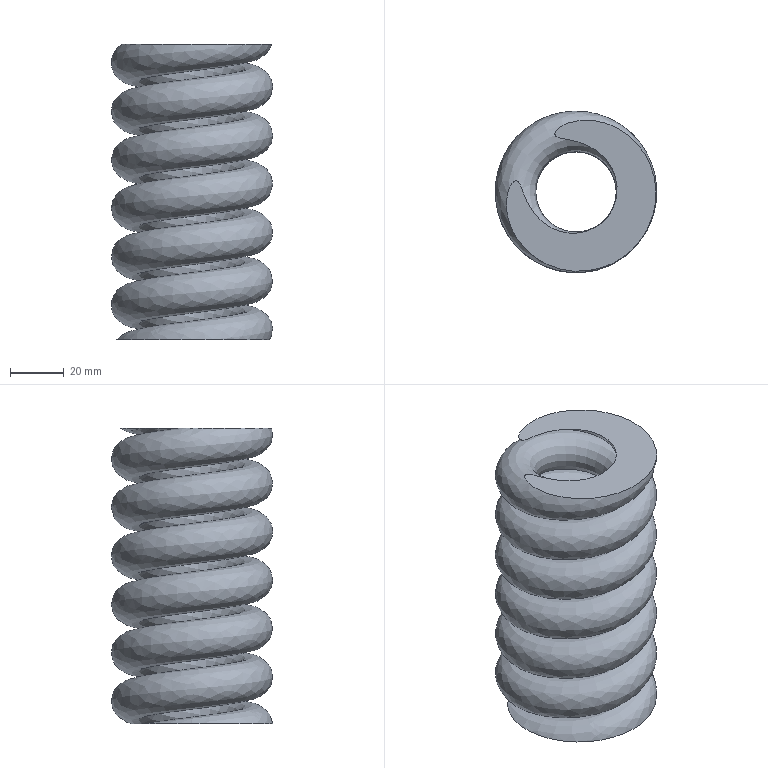Part | NX | features solid 2 | 1 solid | 3 faces | box 60 x 60 x 110 mm | volume 153067 mm3 | plane 2 | spline 1